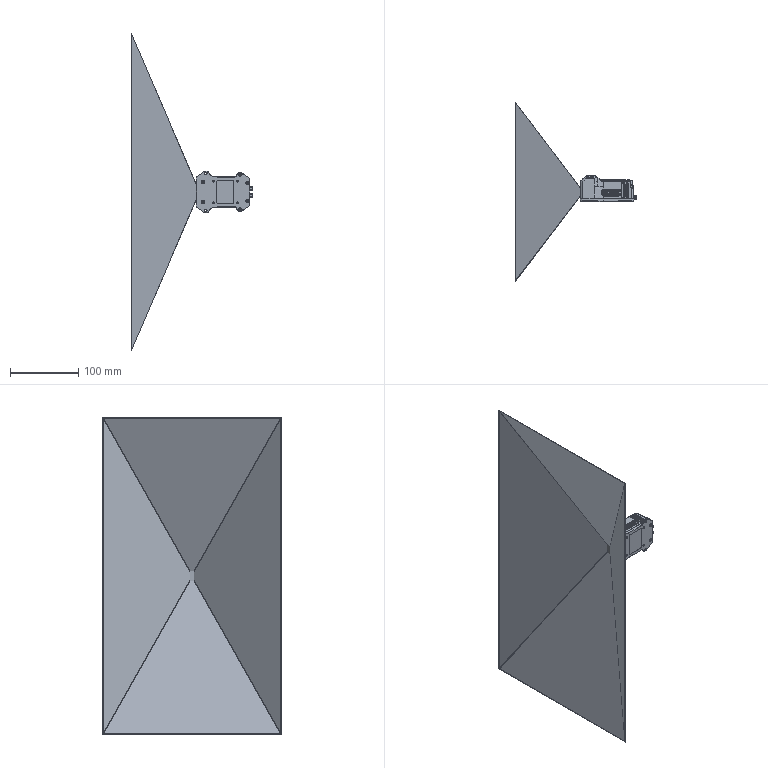Part | SolidWorks | 2 solids | 1532 faces | box 178.016 x 263.013 x 465.513 mm | volume 233417 mm3 | plane 609 | spline 458 | cylinder 337 | cone 98 | torus 30 | commonest cylinder face diameters 0.6 x135 1 x30 4 x28 0.5 x16 2.5 x16 0.4 x13